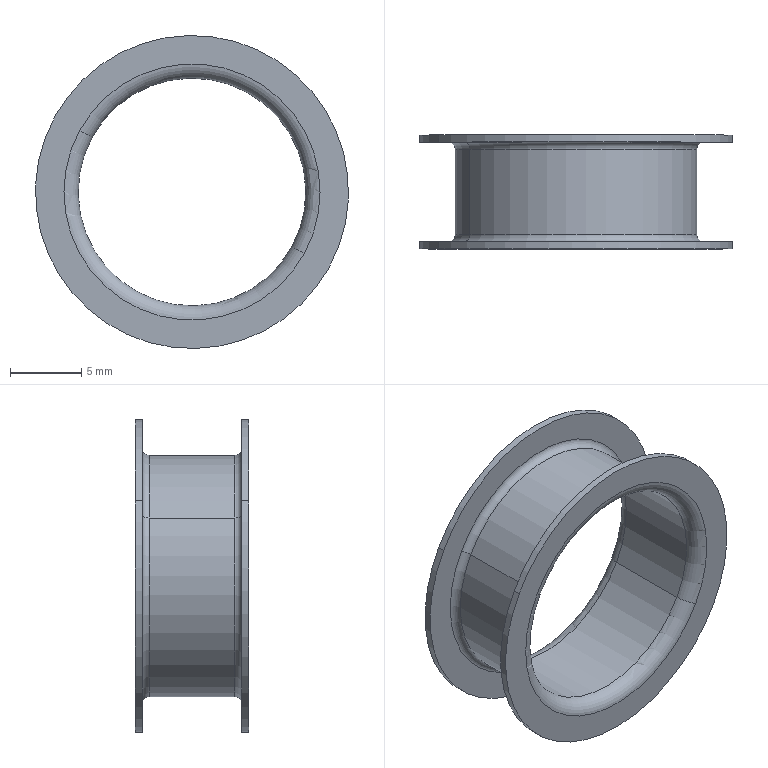Part | NX | features BREP 1 | 1 solid | 20 faces | box 22 x 8 x 22 mm | volume 344.125 mm3 | torus 8 | cylinder 8 | plane 4 | commonest cylinder face diameters 22 x4 16 x2 17 x2
STEP:
#1=CARTESIAN_POINT('',(-7.898,0.,4.315));
#2=VERTEX_POINT('',#1);
#3=CARTESIAN_POINT('',(7.898,0.,-4.315));
#4=VERTEX_POINT('',#3);
#5=CARTESIAN_POINT('',(0.,0.,0.));
#6=DIRECTION('',(0.,1.,0.));
#7=DIRECTION('',(-0.8776,0.,0.4794));
#8=AXIS2_PLACEMENT_3D('',#5,#6,#7);
#9=CIRCLE('',#8,9.);
#10=EDGE_CURVE('',#2,#4,#9,.T.);
#11=ORIENTED_EDGE('',*,*,#10,.F.);
#12=CARTESIAN_POINT('',(-7.021,1.,3.835));
#13=VERTEX_POINT('',#12);
#14=CARTESIAN_POINT('',(-7.898,1.,4.315));
#15=DIRECTION('',(-0.4794,0.,-0.8776));
#16=DIRECTION('',(-0.8776,0.,0.4794));
#17=AXIS2_PLACEMENT_3D('',#14,#15,#16);
#18=CIRCLE('',#17,1.);
#19=EDGE_CURVE('',#2,#13,#18,.F.);
#20=ORIENTED_EDGE('',*,*,#19,.T.);
#21=CARTESIAN_POINT('',(7.021,1.,-3.835));
#22=VERTEX_POINT('',#21);
#23=CARTESIAN_POINT('',(0.,1.,0.));
#24=DIRECTION('',(0.,1.,0.));
#25=DIRECTION('',(-0.8776,0.,0.4794));
#26=AXIS2_PLACEMENT_3D('',#23,#24,#25);
#27=CIRCLE('',#26,8.);
#28=EDGE_CURVE('',#13,#22,#27,.T.);
#29=ORIENTED_EDGE('',*,*,#28,.T.);
#30=CARTESIAN_POINT('',(7.898,1.,-4.315));
#31=DIRECTION('',(0.4794,0.,0.8776));
#32=DIRECTION('',(0.8776,0.,-0.4794));
#33=AXIS2_PLACEMENT_3D('',#30,#31,#32);
#34=CIRCLE('',#33,1.);
#35=EDGE_CURVE('',#4,#22,#34,.F.);
#36=ORIENTED_EDGE('',*,*,#35,.F.);
#37=EDGE_LOOP('',(#11,#20,#29,#36));
#38=FACE_BOUND('',#37,.T.);
#39=CARTESIAN_POINT('',(0.,1.,0.));
#40=DIRECTION('',(0.,1.,0.));
#41=DIRECTION('',(0.8776,0.,-0.4794));
#42=AXIS2_PLACEMENT_3D('',#39,#40,#41);
#43=TOROIDAL_SURFACE('',#42,9.,1.);
#44=ADVANCED_FACE('',(#38),#43,.T.);
#45=CARTESIAN_POINT('',(0.,0.,0.));
#46=DIRECTION('',(0.,1.,0.));
#47=DIRECTION('',(0.8776,0.,-0.4794));
#48=AXIS2_PLACEMENT_3D('',#45,#46,#47);
#49=CIRCLE('',#48,9.);
#50=EDGE_CURVE('',#4,#2,#49,.T.);
#51=ORIENTED_EDGE('',*,*,#50,.F.);
#52=ORIENTED_EDGE('',*,*,#35,.T.);
#53=CARTESIAN_POINT('',(0.,1.,0.));
#54=DIRECTION('',(0.,1.,0.));
#55=DIRECTION('',(0.8776,0.,-0.4794));
#56=AXIS2_PLACEMENT_3D('',#53,#54,#55);
#57=CIRCLE('',#56,8.);
#58=EDGE_CURVE('',#22,#13,#57,.T.);
#59=ORIENTED_EDGE('',*,*,#58,.T.);
#60=ORIENTED_EDGE('',*,*,#19,.F.);
#61=EDGE_LOOP('',(#51,#52,#59,#60));
#62=FACE_BOUND('',#61,.T.);
#63=CARTESIAN_POINT('',(0.,1.,0.));
#64=DIRECTION('',(0.,1.,0.));
#65=DIRECTION('',(-0.8776,0.,0.4794));
#66=AXIS2_PLACEMENT_3D('',#63,#64,#65);
#67=TOROIDAL_SURFACE('',#66,9.,1.);
#68=ADVANCED_FACE('',(#62),#67,.T.);
#69=CARTESIAN_POINT('',(-7.021,7.,3.835));
#70=VERTEX_POINT('',#69);
#71=CARTESIAN_POINT('',(-7.021,1.,3.835));
#72=DIRECTION('',(0.,1.,0.));
#73=VECTOR('',#72,1000.);
#74=LINE('',#71,#73);
#75=EDGE_CURVE('',#13,#70,#74,.T.);
#76=ORIENTED_EDGE('',*,*,#75,.T.);
#77=CARTESIAN_POINT('',(7.021,7.,-3.835));
#78=VERTEX_POINT('',#77);
#79=CARTESIAN_POINT('',(0.,7.,0.));
#80=DIRECTION('',(0.,1.,0.));
#81=DIRECTION('',(-0.8776,0.,0.4794));
#82=AXIS2_PLACEMENT_3D('',#79,#80,#81);
#83=CIRCLE('',#82,8.);
#84=EDGE_CURVE('',#70,#78,#83,.T.);
#85=ORIENTED_EDGE('',*,*,#84,.T.);
#86=CARTESIAN_POINT('',(7.021,1.,-3.835));
#87=DIRECTION('',(0.,1.,0.));
#88=VECTOR('',#87,1000.);
#89=LINE('',#86,#88);
#90=EDGE_CURVE('',#22,#78,#89,.T.);
#91=ORIENTED_EDGE('',*,*,#90,.F.);
#92=ORIENTED_EDGE('',*,*,#28,.F.);
#93=EDGE_LOOP('',(#76,#85,#91,#92));
#94=FACE_BOUND('',#93,.T.);
#95=CARTESIAN_POINT('',(0.,1.,0.));
#96=DIRECTION('',(0.,1.,0.));
#97=DIRECTION('',(0.8776,0.,-0.4794));
#98=AXIS2_PLACEMENT_3D('',#95,#96,#97);
#99=CYLINDRICAL_SURFACE('',#98,8.);
#100=ADVANCED_FACE('',(#94),#99,.F.);
#101=ORIENTED_EDGE('',*,*,#75,.F.);
#102=ORIENTED_EDGE('',*,*,#58,.F.);
#103=ORIENTED_EDGE('',*,*,#90,.T.);
#104=CARTESIAN_POINT('',(0.,7.,0.));
#105=DIRECTION('',(0.,1.,0.));
#106=DIRECTION('',(0.8776,0.,-0.4794));
#107=AXIS2_PLACEMENT_3D('',#104,#105,#106);
#108=CIRCLE('',#107,8.);
#109=EDGE_CURVE('',#78,#70,#108,.T.);
#110=ORIENTED_EDGE('',*,*,#109,.T.);
#111=EDGE_LOOP('',(#101,#102,#103,#110));
#112=FACE_BOUND('',#111,.T.);
#113=CARTESIAN_POINT('',(0.,1.,0.));
#114=DIRECTION('',(0.,1.,0.));
#115=DIRECTION('',(0.8776,0.,-0.4794));
#116=AXIS2_PLACEMENT_3D('',#113,#114,#115);
#117=CYLINDRICAL_SURFACE('',#116,8.);
#118=ADVANCED_FACE('',(#112),#117,.F.);
#119=ORIENTED_EDGE('',*,*,#84,.F.);
#120=CARTESIAN_POINT('',(-7.898,8.,4.315));
#121=VERTEX_POINT('',#120);
#122=CARTESIAN_POINT('',(-7.898,7.,4.315));
#123=DIRECTION('',(-0.4794,0.,-0.8776));
#124=DIRECTION('',(-0.8776,0.,0.4794));
#125=AXIS2_PLACEMENT_3D('',#122,#123,#124);
#126=CIRCLE('',#125,1.);
#127=EDGE_CURVE('',#70,#121,#126,.F.);
#128=ORIENTED_EDGE('',*,*,#127,.T.);
#129=CARTESIAN_POINT('',(7.898,8.,-4.315));
#130=VERTEX_POINT('',#129);
#131=CARTESIAN_POINT('',(0.,8.,0.));
#132=DIRECTION('',(0.,1.,0.));
#133=DIRECTION('',(-0.8776,0.,0.4794));
#134=AXIS2_PLACEMENT_3D('',#131,#132,#133);
#135=CIRCLE('',#134,9.);
#136=EDGE_CURVE('',#121,#130,#135,.T.);
#137=ORIENTED_EDGE('',*,*,#136,.T.);
#138=CARTESIAN_POINT('',(7.898,7.,-4.315));
#139=DIRECTION('',(0.4794,0.,0.8776));
#140=DIRECTION('',(0.8776,0.,-0.4794));
#141=AXIS2_PLACEMENT_3D('',#138,#139,#140);
#142=CIRCLE('',#141,1.);
#143=EDGE_CURVE('',#78,#130,#142,.F.);
#144=ORIENTED_EDGE('',*,*,#143,.F.);
#145=EDGE_LOOP('',(#119,#128,#137,#144));
#146=FACE_BOUND('',#145,.T.);
#147=CARTESIAN_POINT('',(0.,7.,0.));
#148=DIRECTION('',(0.,1.,0.));
#149=DIRECTION('',(0.8776,0.,-0.4794));
#150=AXIS2_PLACEMENT_3D('',#147,#148,#149);
#151=TOROIDAL_SURFACE('',#150,9.,1.);
#152=ADVANCED_FACE('',(#146),#151,.T.);
#153=ORIENTED_EDGE('',*,*,#109,.F.);
#154=ORIENTED_EDGE('',*,*,#143,.T.);
#155=CARTESIAN_POINT('',(0.,8.,0.));
#156=DIRECTION('',(0.,1.,0.));
#157=DIRECTION('',(0.8776,0.,-0.4794));
#158=AXIS2_PLACEMENT_3D('',#155,#156,#157);
#159=CIRCLE('',#158,9.);
#160=EDGE_CURVE('',#130,#121,#159,.T.);
#161=ORIENTED_EDGE('',*,*,#160,.T.);
#162=ORIENTED_EDGE('',*,*,#127,.F.);
#163=EDGE_LOOP('',(#153,#154,#161,#162));
#164=FACE_BOUND('',#163,.T.);
#165=CARTESIAN_POINT('',(0.,7.,0.));
#166=DIRECTION('',(0.,1.,0.));
#167=DIRECTION('',(-0.8776,0.,0.4794));
#168=AXIS2_PLACEMENT_3D('',#165,#166,#167);
#169=TOROIDAL_SURFACE('',#168,9.,1.);
#170=ADVANCED_FACE('',(#164),#169,.T.);
#171=CARTESIAN_POINT('',(-9.653,8.,5.274));
#172=VERTEX_POINT('',#171);
#173=CARTESIAN_POINT('',(-9.653,7.5,5.274));
#174=VERTEX_POINT('',#173);
#175=CARTESIAN_POINT('',(-9.653,8.,5.274));
#176=DIRECTION('',(0.,-1.,0.));
#177=VECTOR('',#176,1000.);
#178=LINE('',#175,#177);
#179=EDGE_CURVE('',#172,#174,#178,.T.);
#180=ORIENTED_EDGE('',*,*,#179,.T.);
#181=CARTESIAN_POINT('',(9.653,7.5,-5.274));
#182=VERTEX_POINT('',#181);
#183=CARTESIAN_POINT('',(0.,7.5,0.));
#184=DIRECTION('',(0.,1.,0.));
#185=DIRECTION('',(-0.8776,0.,0.4794));
#186=AXIS2_PLACEMENT_3D('',#183,#184,#185);
#187=CIRCLE('',#186,11.);
#188=EDGE_CURVE('',#174,#182,#187,.T.);
#189=ORIENTED_EDGE('',*,*,#188,.T.);
#190=CARTESIAN_POINT('',(9.653,8.,-5.274));
#191=VERTEX_POINT('',#190);
#192=CARTESIAN_POINT('',(9.653,8.,-5.274));
#193=DIRECTION('',(0.,-1.,0.));
#194=VECTOR('',#193,1000.);
#195=LINE('',#192,#194);
#196=EDGE_CURVE('',#191,#182,#195,.T.);
#197=ORIENTED_EDGE('',*,*,#196,.F.);
#198=CARTESIAN_POINT('',(0.,8.,0.));
#199=DIRECTION('',(0.,1.,0.));
#200=DIRECTION('',(-0.8776,0.,0.4794));
#201=AXIS2_PLACEMENT_3D('',#198,#199,#200);
#202=CIRCLE('',#201,11.);
#203=EDGE_CURVE('',#172,#191,#202,.T.);
#204=ORIENTED_EDGE('',*,*,#203,.F.);
#205=EDGE_LOOP('',(#180,#189,#197,#204));
#206=FACE_BOUND('',#205,.T.);
#207=CARTESIAN_POINT('',(0.,7.5,0.));
#208=DIRECTION('',(0.,1.,0.));
#209=DIRECTION('',(0.8776,0.,-0.4794));
#210=AXIS2_PLACEMENT_3D('',#207,#208,#209);
#211=CYLINDRICAL_SURFACE('',#210,11.);
#212=ADVANCED_FACE('',(#206),#211,.T.);
#213=ORIENTED_EDGE('',*,*,#179,.F.);
#214=CARTESIAN_POINT('',(0.,8.,0.));
#215=DIRECTION('',(0.,1.,0.));
#216=DIRECTION('',(0.8776,0.,-0.4794));
#217=AXIS2_PLACEMENT_3D('',#214,#215,#216);
#218=CIRCLE('',#217,11.);
#219=EDGE_CURVE('',#191,#172,#218,.T.);
#220=ORIENTED_EDGE('',*,*,#219,.F.);
#221=ORIENTED_EDGE('',*,*,#196,.T.);
#222=CARTESIAN_POINT('',(0.,7.5,0.));
#223=DIRECTION('',(0.,1.,0.));
#224=DIRECTION('',(0.8776,0.,-0.4794));
#225=AXIS2_PLACEMENT_3D('',#222,#223,#224);
#226=CIRCLE('',#225,11.);
#227=EDGE_CURVE('',#182,#174,#226,.T.);
#228=ORIENTED_EDGE('',*,*,#227,.T.);
#229=EDGE_LOOP('',(#213,#220,#221,#228));
#230=FACE_BOUND('',#229,.T.);
#231=CARTESIAN_POINT('',(0.,7.5,0.));
#232=DIRECTION('',(0.,1.,0.));
#233=DIRECTION('',(0.8776,0.,-0.4794));
#234=AXIS2_PLACEMENT_3D('',#231,#232,#233);
#235=CYLINDRICAL_SURFACE('',#234,11.);
#236=ADVANCED_FACE('',(#230),#235,.T.);
#237=CARTESIAN_POINT('',(-7.459,7.,4.075));
#238=VERTEX_POINT('',#237);
#239=CARTESIAN_POINT('',(7.459,7.,-4.075));
#240=VERTEX_POINT('',#239);
#241=CARTESIAN_POINT('',(0.,7.,0.));
#242=DIRECTION('',(0.,1.,0.));
#243=DIRECTION('',(-0.8776,0.,0.4794));
#244=AXIS2_PLACEMENT_3D('',#241,#242,#243);
#245=CIRCLE('',#244,8.5);
#246=EDGE_CURVE('',#238,#240,#245,.T.);
#247=ORIENTED_EDGE('',*,*,#246,.T.);
#248=CARTESIAN_POINT('',(7.898,7.5,-4.315));
#249=VERTEX_POINT('',#248);
#250=CARTESIAN_POINT('',(7.898,7.,-4.315));
#251=DIRECTION('',(0.4794,0.,0.8776));
#252=DIRECTION('',(0.8776,0.,-0.4794));
#253=AXIS2_PLACEMENT_3D('',#250,#251,#252);
#254=CIRCLE('',#253,0.5);
#255=EDGE_CURVE('',#249,#240,#254,.T.);
#256=ORIENTED_EDGE('',*,*,#255,.F.);
#257=CARTESIAN_POINT('',(-7.898,7.5,4.315));
#258=VERTEX_POINT('',#257);
#259=CARTESIAN_POINT('',(0.,7.5,0.));
#260=DIRECTION('',(0.,1.,0.));
#261=DIRECTION('',(-0.8776,0.,0.4794));
#262=AXIS2_PLACEMENT_3D('',#259,#260,#261);
#263=CIRCLE('',#262,9.);
#264=EDGE_CURVE('',#258,#249,#263,.T.);
#265=ORIENTED_EDGE('',*,*,#264,.F.);
#266=CARTESIAN_POINT('',(-7.898,7.,4.315));
#267=DIRECTION('',(-0.4794,0.,-0.8776));
#268=DIRECTION('',(-0.8776,0.,0.4794));
#269=AXIS2_PLACEMENT_3D('',#266,#267,#268);
#270=CIRCLE('',#269,0.5);
#271=EDGE_CURVE('',#258,#238,#270,.T.);
#272=ORIENTED_EDGE('',*,*,#271,.T.);
#273=EDGE_LOOP('',(#247,#256,#265,#272));
#274=FACE_BOUND('',#273,.T.);
#275=CARTESIAN_POINT('',(0.,7.,0.));
#276=DIRECTION('',(0.,1.,0.));
#277=DIRECTION('',(0.8776,0.,-0.4794));
#278=AXIS2_PLACEMENT_3D('',#275,#276,#277);
#279=TOROIDAL_SURFACE('',#278,9.,0.5);
#280=ADVANCED_FACE('',(#274),#279,.F.);
#281=CARTESIAN_POINT('',(0.,7.,0.));
#282=DIRECTION('',(0.,1.,0.));
#283=DIRECTION('',(0.8776,0.,-0.4794));
#284=AXIS2_PLACEMENT_3D('',#281,#282,#283);
#285=CIRCLE('',#284,8.5);
#286=EDGE_CURVE('',#240,#238,#285,.T.);
#287=ORIENTED_EDGE('',*,*,#286,.T.);
#288=ORIENTED_EDGE('',*,*,#271,.F.);
#289=CARTESIAN_POINT('',(0.,7.5,0.));
#290=DIRECTION('',(0.,1.,0.));
#291=DIRECTION('',(0.8776,0.,-0.4794));
#292=AXIS2_PLACEMENT_3D('',#289,#290,#291);
#293=CIRCLE('',#292,9.);
#294=EDGE_CURVE('',#249,#258,#293,.T.);
#295=ORIENTED_EDGE('',*,*,#294,.F.);
#296=ORIENTED_EDGE('',*,*,#255,.T.);
#297=EDGE_LOOP('',(#287,#288,#295,#296));
#298=FACE_BOUND('',#297,.T.);
#299=CARTESIAN_POINT('',(0.,7.,0.));
#300=DIRECTION('',(0.,1.,0.));
#301=DIRECTION('',(-0.8776,0.,0.4794));
#302=AXIS2_PLACEMENT_3D('',#299,#300,#301);
#303=TOROIDAL_SURFACE('',#302,9.,0.5);
#304=ADVANCED_FACE('',(#298),#303,.F.);
#305=CARTESIAN_POINT('',(-7.459,1.,4.075));
#306=VERTEX_POINT('',#305);
#307=CARTESIAN_POINT('',(-7.459,1.,4.075));
#308=DIRECTION('',(0.,1.,0.));
#309=VECTOR('',#308,1000.);
#310=LINE('',#307,#309);
#311=EDGE_CURVE('',#238,#306,#310,.F.);
#312=ORIENTED_EDGE('',*,*,#311,.T.);
#313=CARTESIAN_POINT('',(7.459,1.,-4.075));
#314=VERTEX_POINT('',#313);
#315=CARTESIAN_POINT('',(0.,1.,0.));
#316=DIRECTION('',(0.,1.,0.));
#317=DIRECTION('',(-0.8776,0.,0.4794));
#318=AXIS2_PLACEMENT_3D('',#315,#316,#317);
#319=CIRCLE('',#318,8.5);
#320=EDGE_CURVE('',#306,#314,#319,.T.);
#321=ORIENTED_EDGE('',*,*,#320,.T.);
#322=CARTESIAN_POINT('',(7.459,1.,-4.075));
#323=DIRECTION('',(0.,1.,0.));
#324=VECTOR('',#323,1000.);
#325=LINE('',#322,#324);
#326=EDGE_CURVE('',#240,#314,#325,.F.);
#327=ORIENTED_EDGE('',*,*,#326,.F.);
#328=ORIENTED_EDGE('',*,*,#246,.F.);
#329=EDGE_LOOP('',(#312,#321,#327,#328));
#330=FACE_BOUND('',#329,.T.);
#331=CARTESIAN_POINT('',(0.,1.,0.));
#332=DIRECTION('',(0.,1.,0.));
#333=DIRECTION('',(0.8776,0.,-0.4794));
#334=AXIS2_PLACEMENT_3D('',#331,#332,#333);
#335=CYLINDRICAL_SURFACE('',#334,8.5);
#336=ADVANCED_FACE('',(#330),#335,.T.);
#337=ORIENTED_EDGE('',*,*,#311,.F.);
#338=ORIENTED_EDGE('',*,*,#286,.F.);
#339=ORIENTED_EDGE('',*,*,#326,.T.);
#340=CARTESIAN_POINT('',(0.,1.,0.));
#341=DIRECTION('',(0.,1.,0.));
#342=DIRECTION('',(0.8776,0.,-0.4794));
#343=AXIS2_PLACEMENT_3D('',#340,#341,#342);
#344=CIRCLE('',#343,8.5);
#345=EDGE_CURVE('',#314,#306,#344,.T.);
#346=ORIENTED_EDGE('',*,*,#345,.T.);
#347=EDGE_LOOP('',(#337,#338,#339,#346));
#348=FACE_BOUND('',#347,.T.);
#349=CARTESIAN_POINT('',(0.,1.,0.));
#350=DIRECTION('',(0.,1.,0.));
#351=DIRECTION('',(0.8776,0.,-0.4794));
#352=AXIS2_PLACEMENT_3D('',#349,#350,#351);
#353=CYLINDRICAL_SURFACE('',#352,8.5);
#354=ADVANCED_FACE('',(#348),#353,.T.);
#355=CARTESIAN_POINT('',(-7.898,0.5,4.315));
#356=VERTEX_POINT('',#355);
#357=CARTESIAN_POINT('',(7.898,0.5,-4.315));
#358=VERTEX_POINT('',#357);
#359=CARTESIAN_POINT('',(0.,0.5,0.));
#360=DIRECTION('',(0.,1.,0.));
#361=DIRECTION('',(-0.8776,0.,0.4794));
#362=AXIS2_PLACEMENT_3D('',#359,#360,#361);
#363=CIRCLE('',#362,9.);
#364=EDGE_CURVE('',#356,#358,#363,.T.);
#365=ORIENTED_EDGE('',*,*,#364,.T.);
#366=CARTESIAN_POINT('',(7.898,1.,-4.315));
#367=DIRECTION('',(0.4794,0.,0.8776));
#368=DIRECTION('',(0.8776,0.,-0.4794));
#369=AXIS2_PLACEMENT_3D('',#366,#367,#368);
#370=CIRCLE('',#369,0.5);
#371=EDGE_CURVE('',#314,#358,#370,.T.);
#372=ORIENTED_EDGE('',*,*,#371,.F.);
#373=ORIENTED_EDGE('',*,*,#320,.F.);
#374=CARTESIAN_POINT('',(-7.898,1.,4.315));
#375=DIRECTION('',(-0.4794,0.,-0.8776));
#376=DIRECTION('',(-0.8776,0.,0.4794));
#377=AXIS2_PLACEMENT_3D('',#374,#375,#376);
#378=CIRCLE('',#377,0.5);
#379=EDGE_CURVE('',#306,#356,#378,.T.);
#380=ORIENTED_EDGE('',*,*,#379,.T.);
#381=EDGE_LOOP('',(#365,#372,#373,#380));
#382=FACE_BOUND('',#381,.T.);
#383=CARTESIAN_POINT('',(0.,1.,0.));
#384=DIRECTION('',(0.,1.,0.));
#385=DIRECTION('',(0.8776,0.,-0.4794));
#386=AXIS2_PLACEMENT_3D('',#383,#384,#385);
#387=TOROIDAL_SURFACE('',#386,9.,0.5);
#388=ADVANCED_FACE('',(#382),#387,.F.);
#389=CARTESIAN_POINT('',(0.,0.5,0.));
#390=DIRECTION('',(0.,1.,0.));
#391=DIRECTION('',(0.8776,0.,-0.4794));
#392=AXIS2_PLACEMENT_3D('',#389,#390,#391);
#393=CIRCLE('',#392,9.);
#394=EDGE_CURVE('',#358,#356,#393,.T.);
#395=ORIENTED_EDGE('',*,*,#394,.T.);
#396=ORIENTED_EDGE('',*,*,#379,.F.);
#397=ORIENTED_EDGE('',*,*,#345,.F.);
#398=ORIENTED_EDGE('',*,*,#371,.T.);
#399=EDGE_LOOP('',(#395,#396,#397,#398));
#400=FACE_BOUND('',#399,.T.);
#401=CARTESIAN_POINT('',(0.,1.,0.));
#402=DIRECTION('',(0.,1.,0.));
#403=DIRECTION('',(-0.8776,0.,0.4794));
#404=AXIS2_PLACEMENT_3D('',#401,#402,#403);
#405=TOROIDAL_SURFACE('',#404,9.,0.5);
#406=ADVANCED_FACE('',(#400),#405,.F.);
#407=CARTESIAN_POINT('',(-9.653,0.5,5.274));
#408=VERTEX_POINT('',#407);
#409=CARTESIAN_POINT('',(-9.653,0.,5.274));
#410=VERTEX_POINT('',#409);
#411=CARTESIAN_POINT('',(-9.653,0.5,5.274));
#412=DIRECTION('',(0.,-1.,0.));
#413=VECTOR('',#412,1000.);
#414=LINE('',#411,#413);
#415=EDGE_CURVE('',#408,#410,#414,.T.);
#416=ORIENTED_EDGE('',*,*,#415,.T.);
#417=CARTESIAN_POINT('',(9.653,0.,-5.274));
#418=VERTEX_POINT('',#417);
#419=CARTESIAN_POINT('',(0.,0.,0.));
#420=DIRECTION('',(0.,1.,0.));
#421=DIRECTION('',(-0.8776,0.,0.4794));
#422=AXIS2_PLACEMENT_3D('',#419,#420,#421);
#423=CIRCLE('',#422,11.);
#424=EDGE_CURVE('',#410,#418,#423,.T.);
#425=ORIENTED_EDGE('',*,*,#424,.T.);
#426=CARTESIAN_POINT('',(9.653,0.5,-5.274));
#427=VERTEX_POINT('',#426);
#428=CARTESIAN_POINT('',(9.653,0.5,-5.274));
#429=DIRECTION('',(0.,-1.,0.));
#430=VECTOR('',#429,1000.);
#431=LINE('',#428,#430);
#432=EDGE_CURVE('',#427,#418,#431,.T.);
#433=ORIENTED_EDGE('',*,*,#432,.F.);
#434=CARTESIAN_POINT('',(0.,0.5,0.));
#435=DIRECTION('',(0.,1.,0.));
#436=DIRECTION('',(-0.8776,0.,0.4794));
#437=AXIS2_PLACEMENT_3D('',#434,#435,#436);
#438=CIRCLE('',#437,11.);
#439=EDGE_CURVE('',#408,#427,#438,.T.);
#440=ORIENTED_EDGE('',*,*,#439,.F.);
#441=EDGE_LOOP('',(#416,#425,#433,#440));
#442=FACE_BOUND('',#441,.T.);
#443=CARTESIAN_POINT('',(0.,0.,0.));
#444=DIRECTION('',(0.,1.,0.));
#445=DIRECTION('',(0.8776,0.,-0.4794));
#446=AXIS2_PLACEMENT_3D('',#443,#444,#445);
#447=CYLINDRICAL_SURFACE('',#446,11.);
#448=ADVANCED_FACE('',(#442),#447,.T.);
#449=ORIENTED_EDGE('',*,*,#415,.F.);
#450=CARTESIAN_POINT('',(0.,0.5,0.));
#451=DIRECTION('',(0.,1.,0.));
#452=DIRECTION('',(0.8776,0.,-0.4794));
#453=AXIS2_PLACEMENT_3D('',#450,#451,#452);
#454=CIRCLE('',#453,11.);
#455=EDGE_CURVE('',#427,#408,#454,.T.);
#456=ORIENTED_EDGE('',*,*,#455,.F.);
#457=ORIENTED_EDGE('',*,*,#432,.T.);
#458=CARTESIAN_POINT('',(0.,0.,0.));
#459=DIRECTION('',(0.,1.,0.));
#460=DIRECTION('',(0.8776,0.,-0.4794));
#461=AXIS2_PLACEMENT_3D('',#458,#459,#460);
#462=CIRCLE('',#461,11.);
#463=EDGE_CURVE('',#418,#410,#462,.T.);
#464=ORIENTED_EDGE('',*,*,#463,.T.);
#465=EDGE_LOOP('',(#449,#456,#457,#464));
#466=FACE_BOUND('',#465,.T.);
#467=CARTESIAN_POINT('',(0.,0.,0.));
#468=DIRECTION('',(0.,1.,0.));
#469=DIRECTION('',(0.8776,0.,-0.4794));
#470=AXIS2_PLACEMENT_3D('',#467,#468,#469);
#471=CYLINDRICAL_SURFACE('',#470,11.);
#472=ADVANCED_FACE('',(#466),#471,.T.);
#473=ORIENTED_EDGE('',*,*,#463,.F.);
#474=ORIENTED_EDGE('',*,*,#424,.F.);
#475=EDGE_LOOP('',(#473,#474));
#476=FACE_BOUND('',#475,.T.);
#477=ORIENTED_EDGE('',*,*,#10,.T.);
#478=ORIENTED_EDGE('',*,*,#50,.T.);
#479=EDGE_LOOP('',(#477,#478));
#480=FACE_BOUND('',#479,.T.);
#481=CARTESIAN_POINT('',(-17.913,0.,17.913));
#482=DIRECTION('',(0.,-1.,0.));
#483=DIRECTION('',(0.,0.,1.));
#484=AXIS2_PLACEMENT_3D('',#481,#482,#483);
#485=PLANE('',#484);
#486=ADVANCED_FACE('',(#476,#480),#485,.T.);
#487=ORIENTED_EDGE('',*,*,#219,.T.);
#488=ORIENTED_EDGE('',*,*,#203,.T.);
#489=EDGE_LOOP('',(#487,#488));
#490=FACE_BOUND('',#489,.T.);
#491=ORIENTED_EDGE('',*,*,#136,.F.);
#492=ORIENTED_EDGE('',*,*,#160,.F.);
#493=EDGE_LOOP('',(#491,#492));
#494=FACE_BOUND('',#493,.T.);
#495=CARTESIAN_POINT('',(-17.913,8.,17.913));
#496=DIRECTION('',(0.,1.,0.));
#497=DIRECTION('',(-1.,0.,0.));
#498=AXIS2_PLACEMENT_3D('',#495,#496,#497);
#499=PLANE('',#498);
#500=ADVANCED_FACE('',(#490,#494),#499,.T.);
#501=ORIENTED_EDGE('',*,*,#227,.F.);
#502=ORIENTED_EDGE('',*,*,#188,.F.);
#503=EDGE_LOOP('',(#501,#502));
#504=FACE_BOUND('',#503,.T.);
#505=ORIENTED_EDGE('',*,*,#264,.T.);
#506=ORIENTED_EDGE('',*,*,#294,.T.);
#507=EDGE_LOOP('',(#505,#506));
#508=FACE_BOUND('',#507,.T.);
#509=CARTESIAN_POINT('',(-17.913,7.5,17.913));
#510=DIRECTION('',(0.,-1.,0.));
#511=DIRECTION('',(0.,0.,1.));
#512=AXIS2_PLACEMENT_3D('',#509,#510,#511);
#513=PLANE('',#512);
#514=ADVANCED_FACE('',(#504,#508),#513,.T.);
#515=ORIENTED_EDGE('',*,*,#455,.T.);
#516=ORIENTED_EDGE('',*,*,#439,.T.);
#517=EDGE_LOOP('',(#515,#516));
#518=FACE_BOUND('',#517,.T.);
#519=ORIENTED_EDGE('',*,*,#364,.F.);
#520=ORIENTED_EDGE('',*,*,#394,.F.);
#521=EDGE_LOOP('',(#519,#520));
#522=FACE_BOUND('',#521,.T.);
#523=CARTESIAN_POINT('',(-17.913,0.5,17.913));
#524=DIRECTION('',(0.,1.,0.));
#525=DIRECTION('',(-1.,0.,0.));
#526=AXIS2_PLACEMENT_3D('',#523,#524,#525);
#527=PLANE('',#526);
#528=ADVANCED_FACE('',(#518,#522),#527,.T.);
#529=CLOSED_SHELL('',(#44,#68,#100,#118,#152,#170,#212,#236,#280,#304,#336,#354,#388,#406,#448,#472,#486,#500,#514,#528));
#530=MANIFOLD_SOLID_BREP('',#529);
#531=(LENGTH_UNIT()NAMED_UNIT(*)SI_UNIT(.MILLI.,.METRE.));
#532=UNCERTAINTY_MEASURE_WITH_UNIT(LENGTH_MEASURE(0.00001),#531,'','');
#533=(NAMED_UNIT(*)PLANE_ANGLE_UNIT()SI_UNIT($,.RADIAN.));
#534=(NAMED_UNIT(*)SI_UNIT($,.STERADIAN.)SOLID_ANGLE_UNIT());
#535=(GEOMETRIC_REPRESENTATION_CONTEXT(3)GLOBAL_UNCERTAINTY_ASSIGNED_CONTEXT((#532))GLOBAL_UNIT_ASSIGNED_CONTEXT((#531,#533,#534))REPRESENTATION_CONTEXT('',''));
#536=ADVANCED_BREP_SHAPE_REPRESENTATION('',(#530),#535);